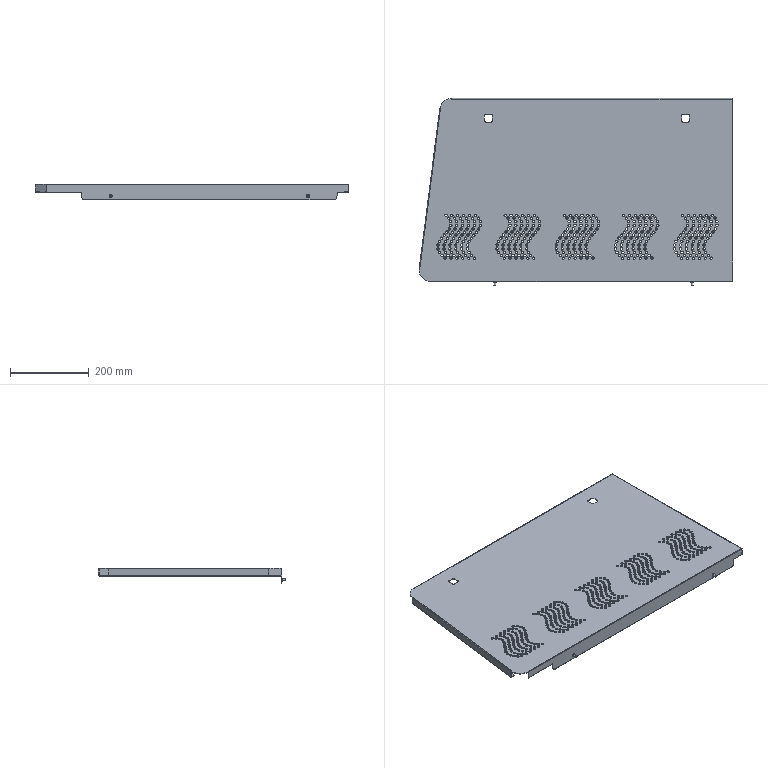Part | STEP file | FHD-021-011-A side door A | 1 solid | 515 faces | box 795.88 x 474.5 x 40 mm | volume 624851 mm3 | cylinder 452 | plane 59 | spline 4 | commonest cylinder face diameters 6 x420 8 x10 0.4 x7 3.4 x7 5.2 x4 20 x2